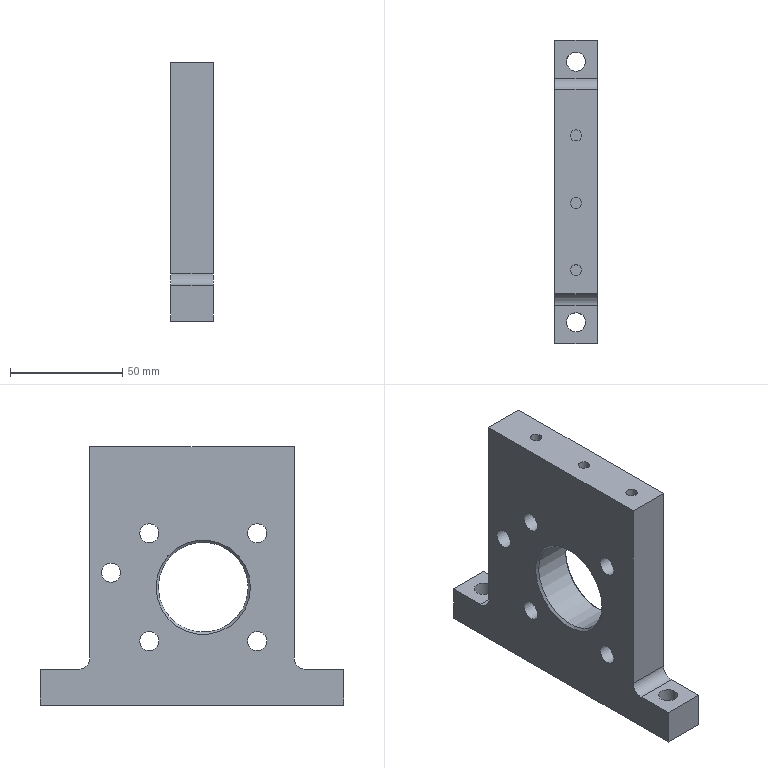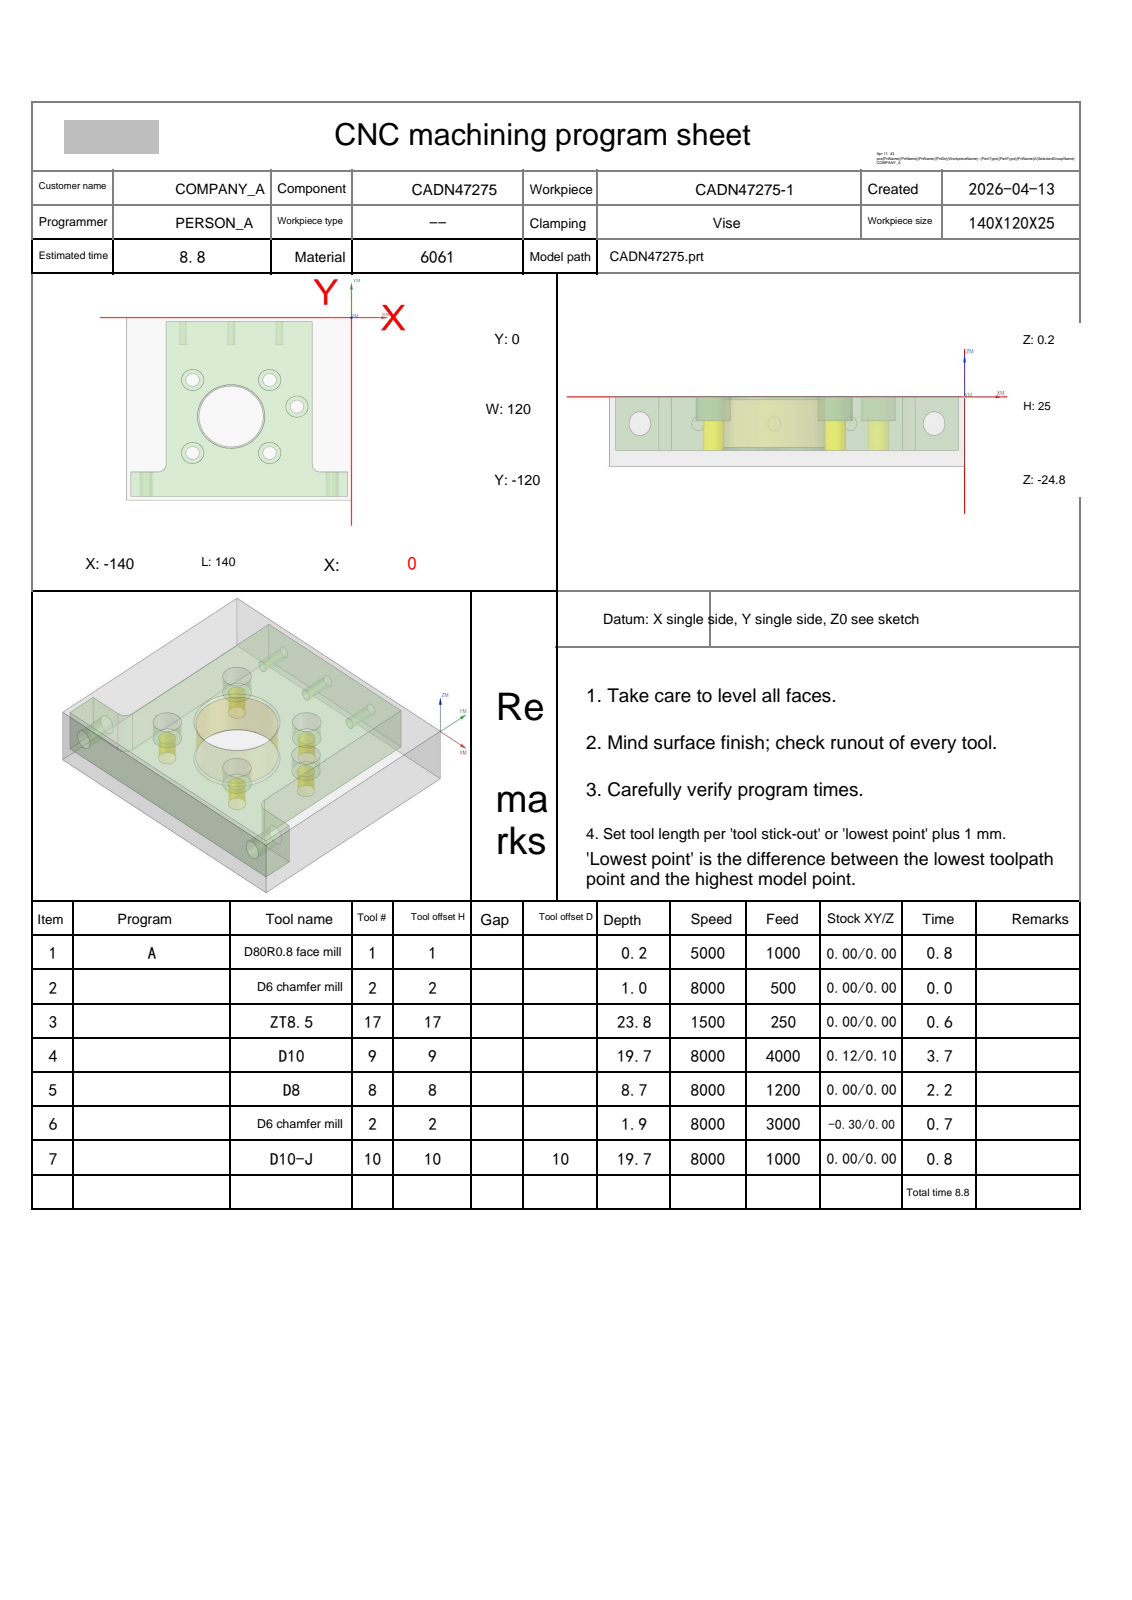NC program | NX | posted by the shop | part box 19 x 135 x 115 mm
Lines 1 to 72 of 2456:
%
O0001
(Machine time: 10.17 MIN)
(===Total Tool:6===)
(T1=D80R0.8 face mill D=80.  R=0.8  D-  H01 Z=-0.   )
(T2=D6 chamfer mill   D=6.   R=0.   D-  H02 Z=-1.7  )
(T17=ZT8.5  D=8.5  DR_a=118 D-  H17 Z=-23.55)
(T9=D10     D=10.  R=0.   D-  H09 Z=-19.5 )
(T8=D8      D=8.   R=0.   D8  H08 Z=-8.5  )
(T10=D10-J  D=10.  R=0.   D10 H10 Z=-19.5 )
G80 G90 G17 G49 G40
G91 G28 Z0
M01
N1 T01 M06
(D80R0.8 face mill  D=80. R=0.8 H=01 ce=0.00 di=0.00)
G00 G90 G54 X-182.5 Y-11.25 M03 S5000
G43 H01 Z20.
M08
Z2.
G01 Z0.0 F1000.
X-177.5
X37.5
Y-60.
X-177.5
Y-108.75
X37.5
X42.5
Z2.
G00 Z20.
G91 G28 Z0.0
M05
M09
G91 G28 Z0.0
M01
N2 T02 M06
(D6 chamfer mill  D=6. R=0. H=02 ce=0.00 di=0.00)
G00 G90 G54 X-99. Y-89. M03 S8000
G43 H02 Z20.
M08
G98 G81 X-99. Y-89. Z-.8 R1. F500.
X-51.
X-34. Y-58.5
X-51. Y-41.
X-99.
X-75. Y-65.
G80
G00 Z20.
G91 G28 Z0.0
M05
M09
G91 G28 Z0.0
M01
N3 T17 M06
(ZT8.5 D=8.5 DR_a=118 H=17)
G00 G90 G54 X-99. Y-89. M03 S1500
G43 H17 Z20.
M08
G98 G83 X-99. Y-89. Z-23.554 R1. F250. Q2.
X-51.
X-34. Y-58.5
X-51. Y-41.
X-99.
X-75. Y-65.
G80
G00 Z20.
G91 G28 Z0.0
M05
M09
G91 G28 Z0.0
M01